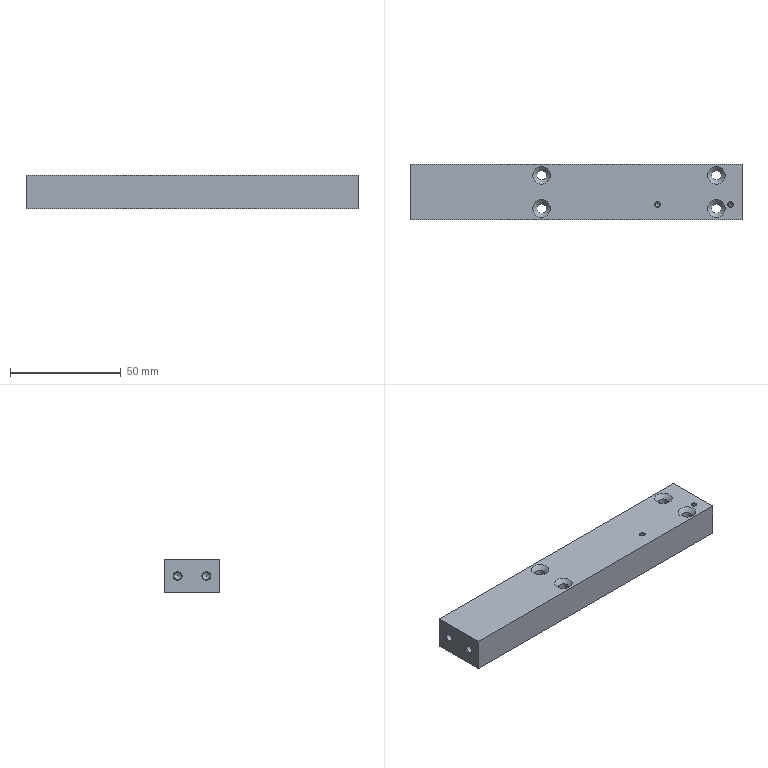Part | STEP file | Chassis spacer strip 1 | 1 solid | 36 faces | box 150 x 25 x 15 mm | volume 54927 mm3 | cone 20 | cylinder 10 | plane 6 | commonest cylinder face diameters 3.3 x4 4.3 x4 2.05 x2